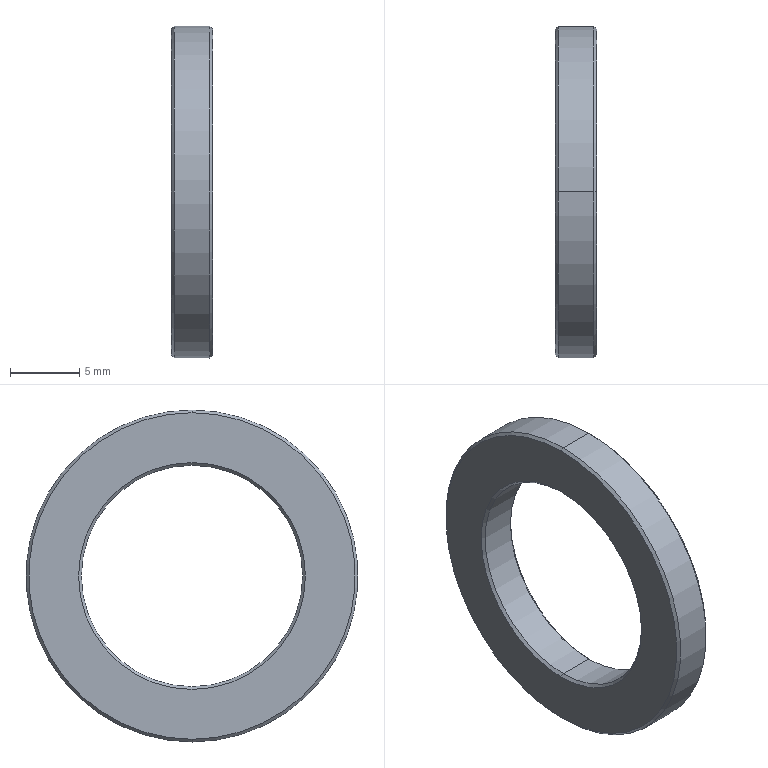Part | STEP file | YOUFENG24X3X16-1 | 1 solid | 14 faces | box 3 x 24 x 24 mm | volume 748.955 mm3 | cone 8 | cylinder 4 | plane 2 | commonest cylinder face diameters 16 x2 24 x2
STEP:
#1=CARTESIAN_POINT('',(0.,0.,0.));
#2=DIRECTION('',(0.,0.,1.));
#3=DIRECTION('',(1.,0.,0.));
#4=AXIS2_PLACEMENT_3D('',#1,#2,#3);
#5=CARTESIAN_POINT('',(19.655,27.,-30.));
#6=VERTEX_POINT('',#5);
#7=CARTESIAN_POINT('',(22.255,27.,-30.));
#8=VERTEX_POINT('',#7);
#9=CARTESIAN_POINT('',(19.655,27.,-30.));
#10=DIRECTION('',(1.,0.,0.));
#11=VECTOR('',#10,1.);
#12=LINE('',#9,#11);
#13=CARTESIAN_POINT('',(19.655,27.,-22.));
#14=DIRECTION('',(1.,0.,0.));
#15=DIRECTION('',(0.,0.,-1.));
#16=AXIS2_PLACEMENT_3D('',#13,#14,#15);
#17=CYLINDRICAL_SURFACE('',#16,8.);
#18=CARTESIAN_POINT('',(6.283,0.));
#19=DIRECTION('',(0.,1.));
#20=VECTOR('',#19,1.);
#21=LINE('',#18,#20);
#22=(GEOMETRIC_REPRESENTATION_CONTEXT(2)PARAMETRIC_REPRESENTATION_CONTEXT()REPRESENTATION_CONTEXT('',''));
#23=DEFINITIONAL_REPRESENTATION('',(#21),#22);
#24=PCURVE('',#17,#23);
#25=CARTESIAN_POINT('',(19.655,27.,-22.));
#26=DIRECTION('',(1.,0.,0.));
#27=DIRECTION('',(0.,0.,-1.));
#28=AXIS2_PLACEMENT_3D('',#25,#26,#27);
#29=CYLINDRICAL_SURFACE('',#28,8.);
#30=CARTESIAN_POINT('',(0.,0.));
#31=DIRECTION('',(0.,1.));
#32=VECTOR('',#31,1.);
#33=LINE('',#30,#32);
#34=(GEOMETRIC_REPRESENTATION_CONTEXT(2)PARAMETRIC_REPRESENTATION_CONTEXT()REPRESENTATION_CONTEXT('',''));
#35=DEFINITIONAL_REPRESENTATION('',(#33),#34);
#36=PCURVE('',#29,#35);
#37=SURFACE_CURVE('',#12,(#24,#36),.PCURVE_S1.);
#38=EDGE_CURVE('',#6,#8,#37,.T.);
#39=ORIENTED_EDGE('',*,*,#38,.T.);
#40=CARTESIAN_POINT('',(22.255,27.,-14.));
#41=VERTEX_POINT('',#40);
#42=CARTESIAN_POINT('',(22.255,27.,-22.));
#43=DIRECTION('',(-1.,0.,0.));
#44=DIRECTION('',(0.,0.,-1.));
#45=AXIS2_PLACEMENT_3D('',#42,#43,#44);
#46=CIRCLE('',#45,8.);
#47=CARTESIAN_POINT('',(6.283,2.6));
#48=DIRECTION('',(-1.,0.));
#49=VECTOR('',#48,1.);
#50=LINE('',#47,#49);
#51=(GEOMETRIC_REPRESENTATION_CONTEXT(2)PARAMETRIC_REPRESENTATION_CONTEXT()REPRESENTATION_CONTEXT('',''));
#52=DEFINITIONAL_REPRESENTATION('',(#50),#51);
#53=PCURVE('',#17,#52);
#54=CARTESIAN_POINT('',(22.255,27.,-22.));
#55=DIRECTION('',(1.,0.,0.));
#56=DIRECTION('',(0.,0.,-1.));
#57=AXIS2_PLACEMENT_3D('',#54,#55,#56);
#58=CONICAL_SURFACE('',#57,8.,0.7854);
#59=CARTESIAN_POINT('',(6.283,-0.000003589));
#60=DIRECTION('',(-1.,0.));
#61=VECTOR('',#60,1.);
#62=LINE('',#59,#61);
#63=(GEOMETRIC_REPRESENTATION_CONTEXT(2)PARAMETRIC_REPRESENTATION_CONTEXT()REPRESENTATION_CONTEXT('',''));
#64=DEFINITIONAL_REPRESENTATION('',(#62),#63);
#65=PCURVE('',#58,#64);
#66=SURFACE_CURVE('',#46,(#53,#65),.PCURVE_S1.);
#67=EDGE_CURVE('',#8,#41,#66,.T.);
#68=ORIENTED_EDGE('',*,*,#67,.T.);
#69=CARTESIAN_POINT('',(19.655,27.,-14.));
#70=VERTEX_POINT('',#69);
#71=CARTESIAN_POINT('',(19.655,27.,-14.));
#72=DIRECTION('',(1.,0.,0.));
#73=VECTOR('',#72,1.);
#74=LINE('',#71,#73);
#75=CARTESIAN_POINT('',(3.142,0.));
#76=DIRECTION('',(0.,1.));
#77=VECTOR('',#76,1.);
#78=LINE('',#75,#77);
#79=(GEOMETRIC_REPRESENTATION_CONTEXT(2)PARAMETRIC_REPRESENTATION_CONTEXT()REPRESENTATION_CONTEXT('',''));
#80=DEFINITIONAL_REPRESENTATION('',(#78),#79);
#81=PCURVE('',#17,#80);
#82=CARTESIAN_POINT('',(3.142,0.));
#83=DIRECTION('',(0.,1.));
#84=VECTOR('',#83,1.);
#85=LINE('',#82,#84);
#86=(GEOMETRIC_REPRESENTATION_CONTEXT(2)PARAMETRIC_REPRESENTATION_CONTEXT()REPRESENTATION_CONTEXT('',''));
#87=DEFINITIONAL_REPRESENTATION('',(#85),#86);
#88=PCURVE('',#29,#87);
#89=SURFACE_CURVE('',#74,(#81,#88),.PCURVE_S1.);
#90=EDGE_CURVE('',#70,#41,#89,.T.);
#91=ORIENTED_EDGE('',*,*,#90,.F.);
#92=CARTESIAN_POINT('',(19.655,27.,-22.));
#93=DIRECTION('',(1.,0.,0.));
#94=DIRECTION('',(0.,0.,1.));
#95=AXIS2_PLACEMENT_3D('',#92,#93,#94);
#96=CIRCLE('',#95,8.);
#97=CARTESIAN_POINT('',(3.142,0.));
#98=DIRECTION('',(1.,0.));
#99=VECTOR('',#98,1.);
#100=LINE('',#97,#99);
#101=(GEOMETRIC_REPRESENTATION_CONTEXT(2)PARAMETRIC_REPRESENTATION_CONTEXT()REPRESENTATION_CONTEXT('',''));
#102=DEFINITIONAL_REPRESENTATION('',(#100),#101);
#103=PCURVE('',#17,#102);
#104=CARTESIAN_POINT('',(19.655,27.,-22.));
#105=DIRECTION('',(-1.,0.,0.));
#106=DIRECTION('',(0.,0.,1.));
#107=AXIS2_PLACEMENT_3D('',#104,#105,#106);
#108=CONICAL_SURFACE('',#107,8.,0.7854);
#109=CARTESIAN_POINT('',(6.283,0.));
#110=DIRECTION('',(-1.,0.));
#111=VECTOR('',#110,1.);
#112=LINE('',#109,#111);
#113=(GEOMETRIC_REPRESENTATION_CONTEXT(2)PARAMETRIC_REPRESENTATION_CONTEXT()REPRESENTATION_CONTEXT('',''));
#114=DEFINITIONAL_REPRESENTATION('',(#112),#113);
#115=PCURVE('',#108,#114);
#116=SURFACE_CURVE('',#96,(#103,#115),.PCURVE_S1.);
#117=EDGE_CURVE('',#70,#6,#116,.T.);
#118=ORIENTED_EDGE('',*,*,#117,.T.);
#119=EDGE_LOOP('',(#39,#68,#91,#118));
#120=FACE_BOUND('',#119,.F.);
#121=ADVANCED_FACE('',(#120),#17,.F.);
#122=CARTESIAN_POINT('',(22.455,27.,-30.2));
#123=VERTEX_POINT('',#122);
#124=CARTESIAN_POINT('',(22.255,27.,-30.));
#125=DIRECTION('',(0.7071,0.,-0.7071));
#126=VECTOR('',#125,1.);
#127=LINE('',#124,#126);
#128=CARTESIAN_POINT('',(6.283,0.));
#129=DIRECTION('',(0.,1.));
#130=VECTOR('',#129,1.);
#131=LINE('',#128,#130);
#132=(GEOMETRIC_REPRESENTATION_CONTEXT(2)PARAMETRIC_REPRESENTATION_CONTEXT()REPRESENTATION_CONTEXT('',''));
#133=DEFINITIONAL_REPRESENTATION('',(#131),#132);
#134=PCURVE('',#58,#133);
#135=CARTESIAN_POINT('',(22.255,27.,-22.));
#136=DIRECTION('',(1.,0.,0.));
#137=DIRECTION('',(0.,0.,-1.));
#138=AXIS2_PLACEMENT_3D('',#135,#136,#137);
#139=CONICAL_SURFACE('',#138,8.,0.7854);
#140=CARTESIAN_POINT('',(0.,0.));
#141=DIRECTION('',(0.,1.));
#142=VECTOR('',#141,1.);
#143=LINE('',#140,#142);
#144=(GEOMETRIC_REPRESENTATION_CONTEXT(2)PARAMETRIC_REPRESENTATION_CONTEXT()REPRESENTATION_CONTEXT('',''));
#145=DEFINITIONAL_REPRESENTATION('',(#143),#144);
#146=PCURVE('',#139,#145);
#147=SURFACE_CURVE('',#127,(#134,#146),.PCURVE_S1.);
#148=EDGE_CURVE('',#8,#123,#147,.T.);
#149=ORIENTED_EDGE('',*,*,#148,.T.);
#150=CARTESIAN_POINT('',(22.455,27.,-13.8));
#151=VERTEX_POINT('',#150);
#152=CARTESIAN_POINT('',(22.455,27.,-22.));
#153=DIRECTION('',(-1.,0.,0.));
#154=DIRECTION('',(0.,0.,-1.));
#155=AXIS2_PLACEMENT_3D('',#152,#153,#154);
#156=CIRCLE('',#155,8.2);
#157=CARTESIAN_POINT('',(6.283,0.2));
#158=DIRECTION('',(-1.,0.));
#159=VECTOR('',#158,1.);
#160=LINE('',#157,#159);
#161=(GEOMETRIC_REPRESENTATION_CONTEXT(2)PARAMETRIC_REPRESENTATION_CONTEXT()REPRESENTATION_CONTEXT('',''));
#162=DEFINITIONAL_REPRESENTATION('',(#160),#161);
#163=PCURVE('',#58,#162);
#164=CARTESIAN_POINT('',(22.455,39.281,-34.272));
#165=DIRECTION('',(1.,0.,0.));
#166=DIRECTION('',(0.,0.,1.));
#167=AXIS2_PLACEMENT_3D('',#164,#165,#166);
#168=PLANE('',#167);
#169=CARTESIAN_POINT('',(4.072,12.281));
#170=CARTESIAN_POINT('',(4.072,26.483));
#171=CARTESIAN_POINT('',(16.372,19.382));
#172=CARTESIAN_POINT('',(28.672,12.281));
#173=CARTESIAN_POINT('',(16.372,5.179));
#174=CARTESIAN_POINT('',(4.072,-1.922));
#175=CARTESIAN_POINT('',(4.072,12.281));
#176=(BOUNDED_CURVE()B_SPLINE_CURVE(2,(#169,#170,#171,#172,#173,#174,#175),.UNSPECIFIED.,.T.,.F.)B_SPLINE_CURVE_WITH_KNOTS((1,2,2,2,2,1),(-2.094,0.,2.094,4.189,6.283,8.378),.UNSPECIFIED.)CURVE()GEOMETRIC_REPRESENTATION_ITEM()RATIONAL_B_SPLINE_CURVE((1.,0.5,1.,0.5,1.,0.5,1.))REPRESENTATION_ITEM(''));
#177=(GEOMETRIC_REPRESENTATION_CONTEXT(2)PARAMETRIC_REPRESENTATION_CONTEXT()REPRESENTATION_CONTEXT('',''));
#178=DEFINITIONAL_REPRESENTATION('',(#176),#177);
#179=PCURVE('',#168,#178);
#180=SURFACE_CURVE('',#156,(#163,#179),.PCURVE_S1.);
#181=EDGE_CURVE('',#123,#151,#180,.T.);
#182=ORIENTED_EDGE('',*,*,#181,.T.);
#183=CARTESIAN_POINT('',(22.255,27.,-14.));
#184=DIRECTION('',(0.7071,0.,0.7071));
#185=VECTOR('',#184,1.);
#186=LINE('',#183,#185);
#187=CARTESIAN_POINT('',(3.142,0.));
#188=DIRECTION('',(0.,1.));
#189=VECTOR('',#188,1.);
#190=LINE('',#187,#189);
#191=(GEOMETRIC_REPRESENTATION_CONTEXT(2)PARAMETRIC_REPRESENTATION_CONTEXT()REPRESENTATION_CONTEXT('',''));
#192=DEFINITIONAL_REPRESENTATION('',(#190),#191);
#193=PCURVE('',#58,#192);
#194=CARTESIAN_POINT('',(3.142,0.));
#195=DIRECTION('',(0.,1.));
#196=VECTOR('',#195,1.);
#197=LINE('',#194,#196);
#198=(GEOMETRIC_REPRESENTATION_CONTEXT(2)PARAMETRIC_REPRESENTATION_CONTEXT()REPRESENTATION_CONTEXT('',''));
#199=DEFINITIONAL_REPRESENTATION('',(#197),#198);
#200=PCURVE('',#139,#199);
#201=SURFACE_CURVE('',#186,(#193,#200),.PCURVE_S1.);
#202=EDGE_CURVE('',#41,#151,#201,.T.);
#203=ORIENTED_EDGE('',*,*,#202,.F.);
#204=ORIENTED_EDGE('',*,*,#67,.F.);
#205=EDGE_LOOP('',(#149,#182,#203,#204));
#206=FACE_BOUND('',#205,.F.);
#207=ADVANCED_FACE('',(#206),#58,.F.);
#208=CARTESIAN_POINT('',(19.455,27.,-13.8));
#209=VERTEX_POINT('',#208);
#210=CARTESIAN_POINT('',(19.655,27.,-14.));
#211=DIRECTION('',(-0.7071,0.,0.7071));
#212=VECTOR('',#211,1.);
#213=LINE('',#210,#212);
#214=CARTESIAN_POINT('',(6.283,0.));
#215=DIRECTION('',(0.,1.));
#216=VECTOR('',#215,1.);
#217=LINE('',#214,#216);
#218=(GEOMETRIC_REPRESENTATION_CONTEXT(2)PARAMETRIC_REPRESENTATION_CONTEXT()REPRESENTATION_CONTEXT('',''));
#219=DEFINITIONAL_REPRESENTATION('',(#217),#218);
#220=PCURVE('',#108,#219);
#221=CARTESIAN_POINT('',(19.655,27.,-22.));
#222=DIRECTION('',(-1.,0.,0.));
#223=DIRECTION('',(0.,0.,1.));
#224=AXIS2_PLACEMENT_3D('',#221,#222,#223);
#225=CONICAL_SURFACE('',#224,8.,0.7854);
#226=CARTESIAN_POINT('',(0.,0.));
#227=DIRECTION('',(0.,1.));
#228=VECTOR('',#227,1.);
#229=LINE('',#226,#228);
#230=(GEOMETRIC_REPRESENTATION_CONTEXT(2)PARAMETRIC_REPRESENTATION_CONTEXT()REPRESENTATION_CONTEXT('',''));
#231=DEFINITIONAL_REPRESENTATION('',(#229),#230);
#232=PCURVE('',#225,#231);
#233=SURFACE_CURVE('',#213,(#220,#232),.PCURVE_S1.);
#234=EDGE_CURVE('',#70,#209,#233,.T.);
#235=ORIENTED_EDGE('',*,*,#234,.T.);
#236=CARTESIAN_POINT('',(19.455,27.,-30.2));
#237=VERTEX_POINT('',#236);
#238=CARTESIAN_POINT('',(19.455,27.,-22.));
#239=DIRECTION('',(1.,0.,0.));
#240=DIRECTION('',(0.,0.,-1.));
#241=AXIS2_PLACEMENT_3D('',#238,#239,#240);
#242=CIRCLE('',#241,8.2);
#243=CARTESIAN_POINT('',(9.425,0.2));
#244=DIRECTION('',(-1.,0.));
#245=VECTOR('',#244,1.);
#246=LINE('',#243,#245);
#247=(GEOMETRIC_REPRESENTATION_CONTEXT(2)PARAMETRIC_REPRESENTATION_CONTEXT()REPRESENTATION_CONTEXT('',''));
#248=DEFINITIONAL_REPRESENTATION('',(#246),#247);
#249=PCURVE('',#108,#248);
#250=CARTESIAN_POINT('',(19.455,39.28,-34.272));
#251=DIRECTION('',(1.,0.,0.));
#252=DIRECTION('',(0.,0.,1.));
#253=AXIS2_PLACEMENT_3D('',#250,#251,#252);
#254=PLANE('',#253);
#255=CARTESIAN_POINT('',(12.272,12.28));
#256=DIRECTION('',(-1.,0.));
#257=AXIS2_PLACEMENT_2D('',#255,#256);
#258=CIRCLE('',#257,8.2);
#259=(GEOMETRIC_REPRESENTATION_CONTEXT(2)PARAMETRIC_REPRESENTATION_CONTEXT()REPRESENTATION_CONTEXT('',''));
#260=DEFINITIONAL_REPRESENTATION('',(#258),#259);
#261=PCURVE('',#254,#260);
#262=SURFACE_CURVE('',#242,(#249,#261),.PCURVE_S1.);
#263=EDGE_CURVE('',#209,#237,#262,.T.);
#264=ORIENTED_EDGE('',*,*,#263,.T.);
#265=CARTESIAN_POINT('',(19.655,27.,-30.));
#266=DIRECTION('',(-0.7071,0.,-0.7071));
#267=VECTOR('',#266,1.);
#268=LINE('',#265,#267);
#269=CARTESIAN_POINT('',(3.142,0.));
#270=DIRECTION('',(0.,1.));
#271=VECTOR('',#270,1.);
#272=LINE('',#269,#271);
#273=(GEOMETRIC_REPRESENTATION_CONTEXT(2)PARAMETRIC_REPRESENTATION_CONTEXT()REPRESENTATION_CONTEXT('',''));
#274=DEFINITIONAL_REPRESENTATION('',(#272),#273);
#275=PCURVE('',#108,#274);
#276=CARTESIAN_POINT('',(3.142,0.));
#277=DIRECTION('',(0.,1.));
#278=VECTOR('',#277,1.);
#279=LINE('',#276,#278);
#280=(GEOMETRIC_REPRESENTATION_CONTEXT(2)PARAMETRIC_REPRESENTATION_CONTEXT()REPRESENTATION_CONTEXT('',''));
#281=DEFINITIONAL_REPRESENTATION('',(#279),#280);
#282=PCURVE('',#225,#281);
#283=SURFACE_CURVE('',#268,(#275,#282),.PCURVE_S1.);
#284=EDGE_CURVE('',#6,#237,#283,.T.);
#285=ORIENTED_EDGE('',*,*,#284,.F.);
#286=ORIENTED_EDGE('',*,*,#117,.F.);
#287=EDGE_LOOP('',(#235,#264,#285,#286));
#288=FACE_BOUND('',#287,.F.);
#289=ADVANCED_FACE('',(#288),#108,.F.);
#290=CARTESIAN_POINT('',(22.455,27.,-10.2));
#291=VERTEX_POINT('',#290);
#292=CARTESIAN_POINT('',(22.455,27.,-33.8));
#293=VERTEX_POINT('',#292);
#294=CARTESIAN_POINT('',(22.455,27.,-22.));
#295=DIRECTION('',(-1.,0.,0.));
#296=DIRECTION('',(0.,0.,1.));
#297=AXIS2_PLACEMENT_3D('',#294,#295,#296);
#298=CIRCLE('',#297,11.8);
#299=CARTESIAN_POINT('',(22.455,27.,-22.));
#300=DIRECTION('',(-1.,0.,0.));
#301=DIRECTION('',(0.,0.,1.));
#302=AXIS2_PLACEMENT_3D('',#299,#300,#301);
#303=CONICAL_SURFACE('',#302,11.8,0.7854);
#304=CARTESIAN_POINT('',(0.,0.));
#305=DIRECTION('',(1.,0.));
#306=VECTOR('',#305,1.);
#307=LINE('',#304,#306);
#308=(GEOMETRIC_REPRESENTATION_CONTEXT(2)PARAMETRIC_REPRESENTATION_CONTEXT()REPRESENTATION_CONTEXT('',''));
#309=DEFINITIONAL_REPRESENTATION('',(#307),#308);
#310=PCURVE('',#303,#309);
#311=CARTESIAN_POINT('',(24.072,12.281));
#312=CARTESIAN_POINT('',(24.072,-8.158));
#313=CARTESIAN_POINT('',(6.372,2.061));
#314=CARTESIAN_POINT('',(-11.328,12.281));
#315=CARTESIAN_POINT('',(6.372,22.5));
#316=CARTESIAN_POINT('',(24.072,32.719));
#317=CARTESIAN_POINT('',(24.072,12.281));
#318=(BOUNDED_CURVE()B_SPLINE_CURVE(2,(#311,#312,#313,#314,#315,#316,#317),.UNSPECIFIED.,.T.,.F.)B_SPLINE_CURVE_WITH_KNOTS((1,2,2,2,2,1),(-2.094,0.,2.094,4.189,6.283,8.378),.UNSPECIFIED.)CURVE()GEOMETRIC_REPRESENTATION_ITEM()RATIONAL_B_SPLINE_CURVE((1.,0.5,1.,0.5,1.,0.5,1.))REPRESENTATION_ITEM(''));
#319=(GEOMETRIC_REPRESENTATION_CONTEXT(2)PARAMETRIC_REPRESENTATION_CONTEXT()REPRESENTATION_CONTEXT('',''));
#320=DEFINITIONAL_REPRESENTATION('',(#318),#319);
#321=PCURVE('',#168,#320);
#322=SURFACE_CURVE('',#298,(#310,#321),.PCURVE_S1.);
#323=EDGE_CURVE('',#291,#293,#322,.T.);
#324=ORIENTED_EDGE('',*,*,#323,.T.);
#325=CARTESIAN_POINT('',(22.255,27.,-34.));
#326=VERTEX_POINT('',#325);
#327=CARTESIAN_POINT('',(22.455,27.,-33.8));
#328=DIRECTION('',(-0.7071,0.,-0.7071));
#329=VECTOR('',#328,1.);
#330=LINE('',#327,#329);
#331=CARTESIAN_POINT('',(3.142,0.));
#332=DIRECTION('',(0.,1.));
#333=VECTOR('',#332,1.);
#334=LINE('',#331,#333);
#335=(GEOMETRIC_REPRESENTATION_CONTEXT(2)PARAMETRIC_REPRESENTATION_CONTEXT()REPRESENTATION_CONTEXT('',''));
#336=DEFINITIONAL_REPRESENTATION('',(#334),#335);
#337=PCURVE('',#303,#336);
#338=CARTESIAN_POINT('',(22.455,27.,-22.));
#339=DIRECTION('',(-1.,0.,0.));
#340=DIRECTION('',(0.,0.,1.));
#341=AXIS2_PLACEMENT_3D('',#338,#339,#340);
#342=CONICAL_SURFACE('',#341,11.8,0.7854);
#343=CARTESIAN_POINT('',(3.142,0.));
#344=DIRECTION('',(0.,1.));
#345=VECTOR('',#344,1.);
#346=LINE('',#343,#345);
#347=(GEOMETRIC_REPRESENTATION_CONTEXT(2)PARAMETRIC_REPRESENTATION_CONTEXT()REPRESENTATION_CONTEXT('',''));
#348=DEFINITIONAL_REPRESENTATION('',(#346),#347);
#349=PCURVE('',#342,#348);
#350=SURFACE_CURVE('',#330,(#337,#349),.PCURVE_S1.);
#351=EDGE_CURVE('',#293,#326,#350,.T.);
#352=ORIENTED_EDGE('',*,*,#351,.T.);
#353=CARTESIAN_POINT('',(22.255,27.,-10.));
#354=VERTEX_POINT('',#353);
#355=CARTESIAN_POINT('',(22.255,27.,-22.));
#356=DIRECTION('',(-1.,0.,0.));
#357=DIRECTION('',(0.,0.,-1.));
#358=AXIS2_PLACEMENT_3D('',#355,#356,#357);
#359=CIRCLE('',#358,12.);
#360=CARTESIAN_POINT('',(-3.142,0.2));
#361=DIRECTION('',(1.,0.));
#362=VECTOR('',#361,1.);
#363=LINE('',#360,#362);
#364=(GEOMETRIC_REPRESENTATION_CONTEXT(2)PARAMETRIC_REPRESENTATION_CONTEXT()REPRESENTATION_CONTEXT('',''));
#365=DEFINITIONAL_REPRESENTATION('',(#363),#364);
#366=PCURVE('',#303,#365);
#367=CARTESIAN_POINT('',(19.655,27.,-22.));
#368=DIRECTION('',(1.,0.,0.));
#369=DIRECTION('',(0.,0.,-1.));
#370=AXIS2_PLACEMENT_3D('',#367,#368,#369);
#371=CYLINDRICAL_SURFACE('',#370,12.);
#372=CARTESIAN_POINT('',(6.283,2.6));
#373=DIRECTION('',(-1.,0.));
#374=VECTOR('',#373,1.);
#375=LINE('',#372,#374);
#376=(GEOMETRIC_REPRESENTATION_CONTEXT(2)PARAMETRIC_REPRESENTATION_CONTEXT()REPRESENTATION_CONTEXT('',''));
#377=DEFINITIONAL_REPRESENTATION('',(#375),#376);
#378=PCURVE('',#371,#377);
#379=SURFACE_CURVE('',#359,(#366,#378),.PCURVE_S1.);
#380=EDGE_CURVE('',#354,#326,#379,.T.);
#381=ORIENTED_EDGE('',*,*,#380,.F.);
#382=CARTESIAN_POINT('',(22.455,27.,-10.2));
#383=DIRECTION('',(-0.7071,0.,0.7071));
#384=VECTOR('',#383,1.);
#385=LINE('',#382,#384);
#386=CARTESIAN_POINT('',(0.,0.));
#387=DIRECTION('',(0.,1.));
#388=VECTOR('',#387,1.);
#389=LINE('',#386,#388);
#390=(GEOMETRIC_REPRESENTATION_CONTEXT(2)PARAMETRIC_REPRESENTATION_CONTEXT()REPRESENTATION_CONTEXT('',''));
#391=DEFINITIONAL_REPRESENTATION('',(#389),#390);
#392=PCURVE('',#303,#391);
#393=CARTESIAN_POINT('',(6.283,0.));
#394=DIRECTION('',(0.,1.));
#395=VECTOR('',#394,1.);
#396=LINE('',#393,#395);
#397=(GEOMETRIC_REPRESENTATION_CONTEXT(2)PARAMETRIC_REPRESENTATION_CONTEXT()REPRESENTATION_CONTEXT('',''));
#398=DEFINITIONAL_REPRESENTATION('',(#396),#397);
#399=PCURVE('',#342,#398);
#400=SURFACE_CURVE('',#385,(#392,#399),.PCURVE_S1.);
#401=EDGE_CURVE('',#291,#354,#400,.T.);
#402=ORIENTED_EDGE('',*,*,#401,.F.);
#403=EDGE_LOOP('',(#324,#352,#381,#402));
#404=FACE_BOUND('',#403,.T.);
#405=ADVANCED_FACE('',(#404),#303,.T.);
#406=CARTESIAN_POINT('',(19.455,27.,-33.8));
#407=VERTEX_POINT('',#406);
#408=CARTESIAN_POINT('',(19.455,27.,-10.2));
#409=VERTEX_POINT('',#408);
#410=CARTESIAN_POINT('',(19.455,27.,-22.));
#411=DIRECTION('',(1.,0.,0.));
#412=DIRECTION('',(0.,0.,-1.));
#413=AXIS2_PLACEMENT_3D('',#410,#411,#412);
#414=CIRCLE('',#413,11.8);
#415=CARTESIAN_POINT('',(19.455,27.,-22.));
#416=DIRECTION('',(1.,0.,0.));
#417=DIRECTION('',(0.,0.,-1.));
#418=AXIS2_PLACEMENT_3D('',#415,#416,#417);
#419=CONICAL_SURFACE('',#418,11.8,0.7854);
#420=CARTESIAN_POINT('',(0.,0.));
#421=DIRECTION('',(1.,0.));
#422=VECTOR('',#421,1.);
#423=LINE('',#420,#422);
#424=(GEOMETRIC_REPRESENTATION_CONTEXT(2)PARAMETRIC_REPRESENTATION_CONTEXT()REPRESENTATION_CONTEXT('',''));
#425=DEFINITIONAL_REPRESENTATION('',(#423),#424);
#426=PCURVE('',#419,#425);
#427=CARTESIAN_POINT('',(12.272,12.28));
#428=DIRECTION('',(-1.,0.));
#429=AXIS2_PLACEMENT_2D('',#427,#428);
#430=CIRCLE('',#429,11.8);
#431=(GEOMETRIC_REPRESENTATION_CONTEXT(2)PARAMETRIC_REPRESENTATION_CONTEXT()REPRESENTATION_CONTEXT('',''));
#432=DEFINITIONAL_REPRESENTATION('',(#430),#431);
#433=PCURVE('',#254,#432);
#434=SURFACE_CURVE('',#414,(#426,#433),.PCURVE_S1.);
#435=EDGE_CURVE('',#407,#409,#434,.T.);
#436=ORIENTED_EDGE('',*,*,#435,.T.);
#437=CARTESIAN_POINT('',(19.655,27.,-10.));
#438=VERTEX_POINT('',#437);
#439=CARTESIAN_POINT('',(19.455,27.,-10.2));
#440=DIRECTION('',(0.7071,0.,0.7071));
#441=VECTOR('',#440,1.);
#442=LINE('',#439,#441);
#443=CARTESIAN_POINT('',(3.142,0.));
#444=DIRECTION('',(0.,1.));
#445=VECTOR('',#444,1.);
#446=LINE('',#443,#445);
#447=(GEOMETRIC_REPRESENTATION_CONTEXT(2)PARAMETRIC_REPRESENTATION_CONTEXT()REPRESENTATION_CONTEXT('',''));
#448=DEFINITIONAL_REPRESENTATION('',(#446),#447);
#449=PCURVE('',#419,#448);
#450=CARTESIAN_POINT('',(19.455,27.,-22.));
#451=DIRECTION('',(1.,0.,0.));
#452=DIRECTION('',(0.,0.,-1.));
#453=AXIS2_PLACEMENT_3D('',#450,#451,#452);
#454=CONICAL_SURFACE('',#453,11.8,0.7854);
#455=CARTESIAN_POINT('',(3.142,0.));
#456=DIRECTION('',(0.,1.));
#457=VECTOR('',#456,1.);
#458=LINE('',#455,#457);
#459=(GEOMETRIC_REPRESENTATION_CONTEXT(2)PARAMETRIC_REPRESENTATION_CONTEXT()REPRESENTATION_CONTEXT('',''));
#460=DEFINITIONAL_REPRESENTATION('',(#458),#459);
#461=PCURVE('',#454,#460);
#462=SURFACE_CURVE('',#442,(#449,#461),.PCURVE_S1.);
#463=EDGE_CURVE('',#409,#438,#462,.T.);
#464=ORIENTED_EDGE('',*,*,#463,.T.);
#465=CARTESIAN_POINT('',(19.655,27.,-34.));
#466=VERTEX_POINT('',#465);
#467=CARTESIAN_POINT('',(19.655,27.,-22.));
#468=DIRECTION('',(1.,0.,0.));
#469=DIRECTION('',(0.,0.,-1.));
#470=AXIS2_PLACEMENT_3D('',#467,#468,#469);
#471=CIRCLE('',#470,12.);
#472=CARTESIAN_POINT('',(0.,0.2));
#473=DIRECTION('',(1.,0.));
#474=VECTOR('',#473,1.);
#475=LINE('',#472,#474);
#476=(GEOMETRIC_REPRESENTATION_CONTEXT(2)PARAMETRIC_REPRESENTATION_CONTEXT()REPRESENTATION_CONTEXT('',''));
#477=DEFINITIONAL_REPRESENTATION('',(#475),#476);
#478=PCURVE('',#419,#477);
#479=CARTESIAN_POINT('',(0.,0.000000298));
#480=DIRECTION('',(1.,0.));
#481=VECTOR('',#480,1.);
#482=LINE('',#479,#481);
#483=(GEOMETRIC_REPRESENTATION_CONTEXT(2)PARAMETRIC_REPRESENTATION_CONTEXT()REPRESENTATION_CONTEXT('',''));
#484=DEFINITIONAL_REPRESENTATION('',(#482),#483);
#485=PCURVE('',#371,#484);
#486=SURFACE_CURVE('',#471,(#478,#485),.PCURVE_S1.);
#487=EDGE_CURVE('',#466,#438,#486,.T.);
#488=ORIENTED_EDGE('',*,*,#487,.F.);
#489=CARTESIAN_POINT('',(19.455,27.,-33.8));
#490=DIRECTION('',(0.7071,0.,-0.7071));
#491=VECTOR('',#490,1.);
#492=LINE('',#489,#491);
#493=CARTESIAN_POINT('',(0.,0.));
#494=DIRECTION('',(0.,1.));
#495=VECTOR('',#494,1.);
#496=LINE('',#493,#495);
#497=(GEOMETRIC_REPRESENTATION_CONTEXT(2)PARAMETRIC_REPRESENTATION_CONTEXT()REPRESENTATION_CONTEXT('',''));
#498=DEFINITIONAL_REPRESENTATION('',(#496),#497);
#499=PCURVE('',#419,#498);
#500=CARTESIAN_POINT('',(6.283,0.));
#501=DIRECTION('',(0.,1.));
#502=VECTOR('',#501,1.);
#503=LINE('',#500,#502);
#504=(GEOMETRIC_REPRESENTATION_CONTEXT(2)PARAMETRIC_REPRESENTATION_CONTEXT()REPRESENTATION_CONTEXT('',''));
#505=DEFINITIONAL_REPRESENTATION('',(#503),#504);
#506=PCURVE('',#454,#505);
#507=SURFACE_CURVE('',#492,(#499,#506),.PCURVE_S1.);
#508=EDGE_CURVE('',#407,#466,#507,.T.);
#509=ORIENTED_EDGE('',*,*,#508,.F.);
#510=EDGE_LOOP('',(#436,#464,#488,#509));
#511=FACE_BOUND('',#510,.T.);
#512=ADVANCED_FACE('',(#511),#419,.T.);
#513=ORIENTED_EDGE('',*,*,#487,.T.);
#514=CARTESIAN_POINT('',(19.655,27.,-10.));
#515=DIRECTION('',(1.,0.,0.));
#516=VECTOR('',#515,1.);
#517=LINE('',#514,#516);
#518=CARTESIAN_POINT('',(3.142,0.));
#519=DIRECTION('',(0.,1.));
#520=VECTOR('',#519,1.);
#521=LINE('',#518,#520);
#522=(GEOMETRIC_REPRESENTATION_CONTEXT(2)PARAMETRIC_REPRESENTATION_CONTEXT()REPRESENTATION_CONTEXT('',''));
#523=DEFINITIONAL_REPRESENTATION('',(#521),#522);
#524=PCURVE('',#371,#523);
#525=CARTESIAN_POINT('',(19.655,27.,-22.));
#526=DIRECTION('',(1.,0.,0.));
#527=DIRECTION('',(0.,0.,-1.));
#528=AXIS2_PLACEMENT_3D('',#525,#526,#527);
#529=CYLINDRICAL_SURFACE('',#528,12.);
#530=CARTESIAN_POINT('',(3.142,0.));
#531=DIRECTION('',(0.,1.));
#532=VECTOR('',#531,1.);
#533=LINE('',#530,#532);
#534=(GEOMETRIC_REPRESENTATION_CONTEXT(2)PARAMETRIC_REPRESENTATION_CONTEXT()REPRESENTATION_CONTEXT('',''));
#535=DEFINITIONAL_REPRESENTATION('',(#533),#534);
#536=PCURVE('',#529,#535);
#537=SURFACE_CURVE('',#517,(#524,#536),.PCURVE_S1.);
#538=EDGE_CURVE('',#438,#354,#537,.T.);
#539=ORIENTED_EDGE('',*,*,#538,.T.);
#540=ORIENTED_EDGE('',*,*,#380,.T.);
#541=CARTESIAN_POINT('',(19.655,27.,-34.));
#542=DIRECTION('',(1.,0.,0.));
#543=VECTOR('',#542,1.);
#544=LINE('',#541,#543);
#545=CARTESIAN_POINT('',(0.,0.));
#546=DIRECTION('',(0.,1.));
#547=VECTOR('',#546,1.);
#548=LINE('',#545,#547);
#549=(GEOMETRIC_REPRESENTATION_CONTEXT(2)PARAMETRIC_REPRESENTATION_CONTEXT()REPRESENTATION_CONTEXT('',''));
#550=DEFINITIONAL_REPRESENTATION('',(#548),#549);
#551=PCURVE('',#371,#550);
#552=CARTESIAN_POINT('',(6.283,0.));
#553=DIRECTION('',(0.,1.));
#554=VECTOR('',#553,1.);
#555=LINE('',#552,#554);
#556=(GEOMETRIC_REPRESENTATION_CONTEXT(2)PARAMETRIC_REPRESENTATION_CONTEXT()REPRESENTATION_CONTEXT('',''));
#557=DEFINITIONAL_REPRESENTATION('',(#555),#556);
#558=PCURVE('',#529,#557);
#559=SURFACE_CURVE('',#544,(#551,#558),.PCURVE_S1.);
#560=EDGE_CURVE('',#466,#326,#559,.T.);
#561=ORIENTED_EDGE('',*,*,#560,.F.);
#562=EDGE_LOOP('',(#513,#539,#540,#561));
#563=FACE_BOUND('',#562,.T.);
#564=ADVANCED_FACE('',(#563),#371,.T.);
#565=CARTESIAN_POINT('',(22.255,27.,-22.));
#566=DIRECTION('',(-1.,0.,0.));
#567=DIRECTION('',(0.,0.,-1.));
#568=AXIS2_PLACEMENT_3D('',#565,#566,#567);
#569=CIRCLE('',#568,8.);
#570=CARTESIAN_POINT('',(6.283,2.6));
#571=DIRECTION('',(-1.,0.));
#572=VECTOR('',#571,1.);
#573=LINE('',#570,#572);
#574=(GEOMETRIC_REPRESENTATION_CONTEXT(2)PARAMETRIC_REPRESENTATION_CONTEXT()REPRESENTATION_CONTEXT('',''));
#575=DEFINITIONAL_REPRESENTATION('',(#573),#574);
#576=PCURVE('',#29,#575);
#577=CARTESIAN_POINT('',(6.283,-0.000003589));
#578=DIRECTION('',(-1.,0.));
#579=VECTOR('',#578,1.);
#580=LINE('',#577,#579);
#581=(GEOMETRIC_REPRESENTATION_CONTEXT(2)PARAMETRIC_REPRESENTATION_CONTEXT()REPRESENTATION_CONTEXT('',''));
#582=DEFINITIONAL_REPRESENTATION('',(#580),#581);
#583=PCURVE('',#139,#582);
#584=SURFACE_CURVE('',#569,(#576,#583),.PCURVE_S1.);
#585=EDGE_CURVE('',#41,#8,#584,.T.);
#586=ORIENTED_EDGE('',*,*,#585,.T.);
#587=ORIENTED_EDGE('',*,*,#38,.F.);
#588=CARTESIAN_POINT('',(19.655,27.,-22.));
#589=DIRECTION('',(1.,0.,0.));
#590=DIRECTION('',(0.,0.,1.));
#591=AXIS2_PLACEMENT_3D('',#588,#589,#590);
#592=CIRCLE('',#591,8.);
#593=CARTESIAN_POINT('',(-3.142,0.));
#594=DIRECTION('',(1.,0.));
#595=VECTOR('',#594,1.);
#596=LINE('',#593,#595);
#597=(GEOMETRIC_REPRESENTATION_CONTEXT(2)PARAMETRIC_REPRESENTATION_CONTEXT()REPRESENTATION_CONTEXT('',''));
#598=DEFINITIONAL_REPRESENTATION('',(#596),#597);
#599=PCURVE('',#29,#598);
#600=CARTESIAN_POINT('',(6.283,0.));
#601=DIRECTION('',(-1.,0.));
#602=VECTOR('',#601,1.);
#603=LINE('',#600,#602);
#604=(GEOMETRIC_REPRESENTATION_CONTEXT(2)PARAMETRIC_REPRESENTATION_CONTEXT()REPRESENTATION_CONTEXT('',''));
#605=DEFINITIONAL_REPRESENTATION('',(#603),#604);
#606=PCURVE('',#225,#605);
#607=SURFACE_CURVE('',#592,(#599,#606),.PCURVE_S1.);
#608=EDGE_CURVE('',#6,#70,#607,.T.);
#609=ORIENTED_EDGE('',*,*,#608,.T.);
#610=ORIENTED_EDGE('',*,*,#90,.T.);
#611=EDGE_LOOP('',(#586,#587,#609,#610));
#612=FACE_BOUND('',#611,.F.);
#613=ADVANCED_FACE('',(#612),#29,.F.);
#614=CARTESIAN_POINT('',(22.455,27.,-22.));
#615=DIRECTION('',(-1.,0.,0.));
#616=DIRECTION('',(0.,0.,-1.));
#617=AXIS2_PLACEMENT_3D('',#614,#615,#616);
#618=CIRCLE('',#617,8.2);
#619=CARTESIAN_POINT('',(6.283,0.2));
#620=DIRECTION('',(-1.,0.));
#621=VECTOR('',#620,1.);
#622=LINE('',#619,#621);
#623=(GEOMETRIC_REPRESENTATION_CONTEXT(2)PARAMETRIC_REPRESENTATION_CONTEXT()REPRESENTATION_CONTEXT('',''));
#624=DEFINITIONAL_REPRESENTATION('',(#622),#623);
#625=PCURVE('',#139,#624);
#626=CARTESIAN_POINT('',(4.072,12.281));
#627=CARTESIAN_POINT('',(4.072,26.483));
#628=CARTESIAN_POINT('',(16.372,19.382));
#629=CARTESIAN_POINT('',(28.672,12.281));
#630=CARTESIAN_POINT('',(16.372,5.179));
#631=CARTESIAN_POINT('',(4.072,-1.922));
#632=CARTESIAN_POINT('',(4.072,12.281));
#633=(BOUNDED_CURVE()B_SPLINE_CURVE(2,(#626,#627,#628,#629,#630,#631,#632),.UNSPECIFIED.,.T.,.F.)B_SPLINE_CURVE_WITH_KNOTS((1,2,2,2,2,1),(-2.094,0.,2.094,4.189,6.283,8.378),.UNSPECIFIED.)CURVE()GEOMETRIC_REPRESENTATION_ITEM()RATIONAL_B_SPLINE_CURVE((1.,0.5,1.,0.5,1.,0.5,1.))REPRESENTATION_ITEM(''));
#634=(GEOMETRIC_REPRESENTATION_CONTEXT(2)PARAMETRIC_REPRESENTATION_CONTEXT()REPRESENTATION_CONTEXT('',''));
#635=DEFINITIONAL_REPRESENTATION('',(#633),#634);
#636=PCURVE('',#168,#635);
#637=SURFACE_CURVE('',#618,(#625,#636),.PCURVE_S1.);
#638=EDGE_CURVE('',#151,#123,#637,.T.);
#639=ORIENTED_EDGE('',*,*,#638,.T.);
#640=ORIENTED_EDGE('',*,*,#148,.F.);
#641=ORIENTED_EDGE('',*,*,#585,.F.);
#642=ORIENTED_EDGE('',*,*,#202,.T.);
#643=EDGE_LOOP('',(#639,#640,#641,#642));
#644=FACE_BOUND('',#643,.F.);
#645=ADVANCED_FACE('',(#644),#139,.F.);
#646=CARTESIAN_POINT('',(19.455,27.,-22.));
#647=DIRECTION('',(1.,0.,0.));
#648=DIRECTION('',(0.,0.,-1.));
#649=AXIS2_PLACEMENT_3D('',#646,#647,#648);
#650=CIRCLE('',#649,8.2);
#651=CARTESIAN_POINT('',(3.142,0.2));
#652=DIRECTION('',(-1.,0.));
#653=VECTOR('',#652,1.);
#654=LINE('',#651,#653);
#655=(GEOMETRIC_REPRESENTATION_CONTEXT(2)PARAMETRIC_REPRESENTATION_CONTEXT()REPRESENTATION_CONTEXT('',''));
#656=DEFINITIONAL_REPRESENTATION('',(#654),#655);
#657=PCURVE('',#225,#656);
#658=CARTESIAN_POINT('',(12.272,12.28));
#659=DIRECTION('',(-1.,0.));
#660=AXIS2_PLACEMENT_2D('',#658,#659);
#661=CIRCLE('',#660,8.2);
#662=(GEOMETRIC_REPRESENTATION_CONTEXT(2)PARAMETRIC_REPRESENTATION_CONTEXT()REPRESENTATION_CONTEXT('',''));
#663=DEFINITIONAL_REPRESENTATION('',(#661),#662);
#664=PCURVE('',#254,#663);
#665=SURFACE_CURVE('',#650,(#657,#664),.PCURVE_S1.);
#666=EDGE_CURVE('',#237,#209,#665,.T.);
#667=ORIENTED_EDGE('',*,*,#666,.T.);
#668=ORIENTED_EDGE('',*,*,#234,.F.);
#669=ORIENTED_EDGE('',*,*,#608,.F.);
#670=ORIENTED_EDGE('',*,*,#284,.T.);
#671=EDGE_LOOP('',(#667,#668,#669,#670));
#672=FACE_BOUND('',#671,.F.);
#673=ADVANCED_FACE('',(#672),#225,.F.);
#674=ORIENTED_EDGE('',*,*,#181,.T.);
#675=ORIENTED_EDGE('',*,*,#638,.T.);
#676=EDGE_LOOP('',(#674,#675));
#677=FACE_BOUND('',#676,.T.);
#678=ORIENTED_EDGE('',*,*,#323,.F.);
#679=CARTESIAN_POINT('',(22.455,27.,-22.));
#680=DIRECTION('',(-1.,0.,0.));
#681=DIRECTION('',(0.,0.,1.));
#682=AXIS2_PLACEMENT_3D('',#679,#680,#681);
#683=CIRCLE('',#682,11.8);
#684=CARTESIAN_POINT('',(24.072,12.281));
#685=CARTESIAN_POINT('',(24.072,-8.158));
#686=CARTESIAN_POINT('',(6.372,2.061));
#687=CARTESIAN_POINT('',(-11.328,12.281));
#688=CARTESIAN_POINT('',(6.372,22.5));
#689=CARTESIAN_POINT('',(24.072,32.719));
#690=CARTESIAN_POINT('',(24.072,12.281));
#691=(BOUNDED_CURVE()B_SPLINE_CURVE(2,(#684,#685,#686,#687,#688,#689,#690),.UNSPECIFIED.,.T.,.F.)B_SPLINE_CURVE_WITH_KNOTS((1,2,2,2,2,1),(-2.094,0.,2.094,4.189,6.283,8.378),.UNSPECIFIED.)CURVE()GEOMETRIC_REPRESENTATION_ITEM()RATIONAL_B_SPLINE_CURVE((1.,0.5,1.,0.5,1.,0.5,1.))REPRESENTATION_ITEM(''));
#692=(GEOMETRIC_REPRESENTATION_CONTEXT(2)PARAMETRIC_REPRESENTATION_CONTEXT()REPRESENTATION_CONTEXT('',''));
#693=DEFINITIONAL_REPRESENTATION('',(#691),#692);
#694=PCURVE('',#168,#693);
#695=CARTESIAN_POINT('',(0.,0.));
#696=DIRECTION('',(1.,0.));
#697=VECTOR('',#696,1.);
#698=LINE('',#695,#697);
#699=(GEOMETRIC_REPRESENTATION_CONTEXT(2)PARAMETRIC_REPRESENTATION_CONTEXT()REPRESENTATION_CONTEXT('',''));
#700=DEFINITIONAL_REPRESENTATION('',(#698),#699);
#701=PCURVE('',#342,#700);
#702=SURFACE_CURVE('',#683,(#694,#701),.PCURVE_S1.);
#703=EDGE_CURVE('',#293,#291,#702,.T.);
#704=ORIENTED_EDGE('',*,*,#703,.F.);
#705=EDGE_LOOP('',(#678,#704));
#706=FACE_BOUND('',#705,.T.);
#707=ADVANCED_FACE('',(#677,#706),#168,.T.);
#708=ORIENTED_EDGE('',*,*,#263,.T.);
#709=ORIENTED_EDGE('',*,*,#666,.T.);
#710=EDGE_LOOP('',(#708,#709));
#711=FACE_BOUND('',#710,.T.);
#712=CARTESIAN_POINT('',(19.455,27.,-22.));
#713=DIRECTION('',(1.,0.,0.));
#714=DIRECTION('',(0.,0.,-1.));
#715=AXIS2_PLACEMENT_3D('',#712,#713,#714);
#716=CIRCLE('',#715,11.8);
#717=CARTESIAN_POINT('',(12.272,12.28));
#718=DIRECTION('',(-1.,0.));
#719=AXIS2_PLACEMENT_2D('',#717,#718);
#720=CIRCLE('',#719,11.8);
#721=(GEOMETRIC_REPRESENTATION_CONTEXT(2)PARAMETRIC_REPRESENTATION_CONTEXT()REPRESENTATION_CONTEXT('',''));
#722=DEFINITIONAL_REPRESENTATION('',(#720),#721);
#723=PCURVE('',#254,#722);
#724=CARTESIAN_POINT('',(0.,0.));
#725=DIRECTION('',(1.,0.));
#726=VECTOR('',#725,1.);
#727=LINE('',#724,#726);
#728=(GEOMETRIC_REPRESENTATION_CONTEXT(2)PARAMETRIC_REPRESENTATION_CONTEXT()REPRESENTATION_CONTEXT('',''));
#729=DEFINITIONAL_REPRESENTATION('',(#727),#728);
#730=PCURVE('',#454,#729);
#731=SURFACE_CURVE('',#716,(#723,#730),.PCURVE_S1.);
#732=EDGE_CURVE('',#409,#407,#731,.T.);
#733=ORIENTED_EDGE('',*,*,#732,.T.);
#734=ORIENTED_EDGE('',*,*,#435,.T.);
#735=EDGE_LOOP('',(#733,#734));
#736=FACE_BOUND('',#735,.F.);
#737=ADVANCED_FACE('',(#711,#736),#254,.F.);
#738=ORIENTED_EDGE('',*,*,#351,.F.);
#739=ORIENTED_EDGE('',*,*,#703,.T.);
#740=ORIENTED_EDGE('',*,*,#401,.T.);
#741=CARTESIAN_POINT('',(22.255,27.,-22.));
#742=DIRECTION('',(-1.,0.,0.));
#743=DIRECTION('',(0.,0.,-1.));
#744=AXIS2_PLACEMENT_3D('',#741,#742,#743);
#745=CIRCLE('',#744,12.);
#746=CARTESIAN_POINT('',(3.142,0.2));
#747=DIRECTION('',(1.,0.));
#748=VECTOR('',#747,1.);
#749=LINE('',#746,#748);
#750=(GEOMETRIC_REPRESENTATION_CONTEXT(2)PARAMETRIC_REPRESENTATION_CONTEXT()REPRESENTATION_CONTEXT('',''));
#751=DEFINITIONAL_REPRESENTATION('',(#749),#750);
#752=PCURVE('',#342,#751);
#753=CARTESIAN_POINT('',(6.283,2.6));
#754=DIRECTION('',(-1.,0.));
#755=VECTOR('',#754,1.);
#756=LINE('',#753,#755);
#757=(GEOMETRIC_REPRESENTATION_CONTEXT(2)PARAMETRIC_REPRESENTATION_CONTEXT()REPRESENTATION_CONTEXT('',''));
#758=DEFINITIONAL_REPRESENTATION('',(#756),#757);
#759=PCURVE('',#529,#758);
#760=SURFACE_CURVE('',#745,(#752,#759),.PCURVE_S1.);
#761=EDGE_CURVE('',#326,#354,#760,.T.);
#762=ORIENTED_EDGE('',*,*,#761,.F.);
#763=EDGE_LOOP('',(#738,#739,#740,#762));
#764=FACE_BOUND('',#763,.T.);
#765=ADVANCED_FACE('',(#764),#342,.T.);
#766=ORIENTED_EDGE('',*,*,#463,.F.);
#767=ORIENTED_EDGE('',*,*,#732,.T.);
#768=ORIENTED_EDGE('',*,*,#508,.T.);
#769=CARTESIAN_POINT('',(19.655,27.,-22.));
#770=DIRECTION('',(1.,0.,0.));
#771=DIRECTION('',(0.,0.,-1.));
#772=AXIS2_PLACEMENT_3D('',#769,#770,#771);
#773=CIRCLE('',#772,12.);
#774=CARTESIAN_POINT('',(0.,0.2));
#775=DIRECTION('',(1.,0.));
#776=VECTOR('',#775,1.);
#777=LINE('',#774,#776);
#778=(GEOMETRIC_REPRESENTATION_CONTEXT(2)PARAMETRIC_REPRESENTATION_CONTEXT()REPRESENTATION_CONTEXT('',''));
#779=DEFINITIONAL_REPRESENTATION('',(#777),#778);
#780=PCURVE('',#454,#779);
#781=CARTESIAN_POINT('',(0.,0.000000298));
#782=DIRECTION('',(1.,0.));
#783=VECTOR('',#782,1.);
#784=LINE('',#781,#783);
#785=(GEOMETRIC_REPRESENTATION_CONTEXT(2)PARAMETRIC_REPRESENTATION_CONTEXT()REPRESENTATION_CONTEXT('',''));
#786=DEFINITIONAL_REPRESENTATION('',(#784),#785);
#787=PCURVE('',#529,#786);
#788=SURFACE_CURVE('',#773,(#780,#787),.PCURVE_S1.);
#789=EDGE_CURVE('',#438,#466,#788,.T.);
#790=ORIENTED_EDGE('',*,*,#789,.F.);
#791=EDGE_LOOP('',(#766,#767,#768,#790));
#792=FACE_BOUND('',#791,.T.);
#793=ADVANCED_FACE('',(#792),#454,.T.);
#794=ORIENTED_EDGE('',*,*,#538,.F.);
#795=ORIENTED_EDGE('',*,*,#789,.T.);
#796=ORIENTED_EDGE('',*,*,#560,.T.);
#797=ORIENTED_EDGE('',*,*,#761,.T.);
#798=EDGE_LOOP('',(#794,#795,#796,#797));
#799=FACE_BOUND('',#798,.T.);
#800=ADVANCED_FACE('',(#799),#529,.T.);
#801=CLOSED_SHELL('',(#121,#207,#289,#405,#512,#564,#613,#645,#673,#707,#737,#765,#793,#800));
#802=MANIFOLD_SOLID_BREP('',#801);
#803=(LENGTH_UNIT()NAMED_UNIT(*)SI_UNIT(.MILLI.,.METRE.));
#804=UNCERTAINTY_MEASURE_WITH_UNIT(LENGTH_MEASURE(0.000001),#803,'','');
#805=(NAMED_UNIT(*)PLANE_ANGLE_UNIT()SI_UNIT($,.RADIAN.));
#806=(NAMED_UNIT(*)SI_UNIT($,.STERADIAN.)SOLID_ANGLE_UNIT());
#807=(GEOMETRIC_REPRESENTATION_CONTEXT(3)GLOBAL_UNCERTAINTY_ASSIGNED_CONTEXT((#804))GLOBAL_UNIT_ASSIGNED_CONTEXT((#803,#805,#806))REPRESENTATION_CONTEXT('',''));
#808=ADVANCED_BREP_SHAPE_REPRESENTATION('',(#4,#802),#807);